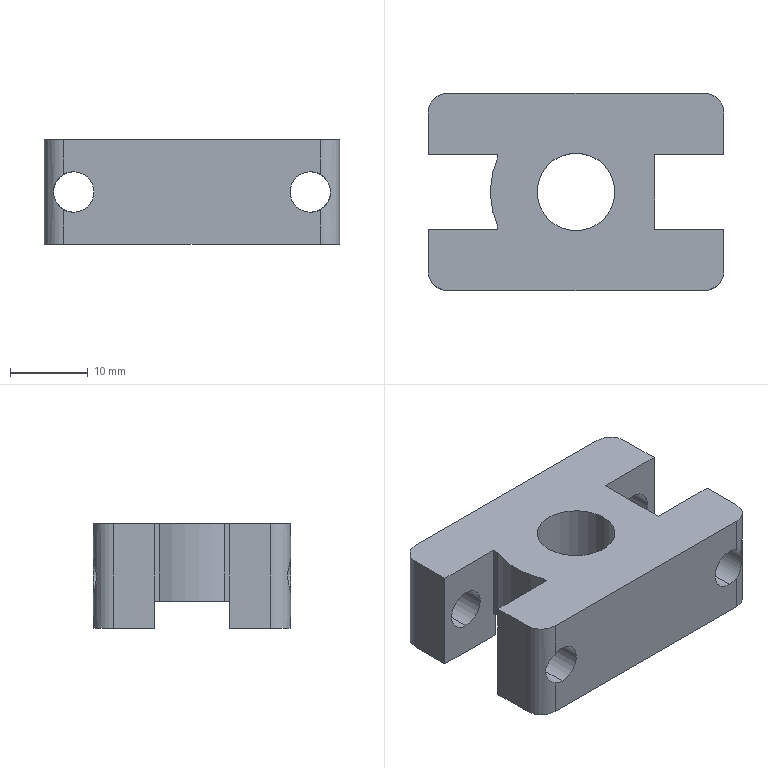Part | SolidWorks | features Cut 2, ICE 2, Extrusion 1, Fillet 1 | 1 solid | 34 faces | box 38.1 x 25.4 x 13.5 mm | volume 7968 mm3 | cylinder 17 | plane 17 | commonest cylinder face diameters 5.207 x8 5.08 x4 22 x3 10 x2
STEP:
#1=CARTESIAN_POINT('',(-15.24,-12.7,0.6465));
#2=VERTEX_POINT('',#1);
#3=CARTESIAN_POINT('',(-16.51,-12.7,0.9773));
#4=VERTEX_POINT('',#3);
#5=CARTESIAN_POINT('',(-15.24,-12.7,3.25));
#6=DIRECTION('',(0.,1.,0.));
#7=DIRECTION('',(0.,0.,1.));
#8=AXIS2_PLACEMENT_3D('',#5,#6,#7);
#9=CIRCLE('',#8,2.604);
#10=EDGE_CURVE('',#2,#4,#9,.T.);
#11=ORIENTED_EDGE('',*,*,#10,.F.);
#12=CARTESIAN_POINT('',(-15.24,-4.826,0.6465));
#13=VERTEX_POINT('',#12);
#14=CARTESIAN_POINT('',(-15.24,-12.7,0.6465));
#15=DIRECTION('',(0.,1.,0.));
#16=VECTOR('',#15,1000.);
#17=LINE('',#14,#16);
#18=EDGE_CURVE('',#2,#13,#17,.T.);
#19=ORIENTED_EDGE('',*,*,#18,.T.);
#20=CARTESIAN_POINT('',(-15.24,-4.826,5.853));
#21=VERTEX_POINT('',#20);
#22=CARTESIAN_POINT('',(-15.24,-4.826,3.25));
#23=DIRECTION('',(0.,1.,0.));
#24=DIRECTION('',(0.,0.,1.));
#25=AXIS2_PLACEMENT_3D('',#22,#23,#24);
#26=CIRCLE('',#25,2.604);
#27=EDGE_CURVE('',#13,#21,#26,.T.);
#28=ORIENTED_EDGE('',*,*,#27,.T.);
#29=CARTESIAN_POINT('',(-15.24,-12.7,5.853));
#30=VERTEX_POINT('',#29);
#31=CARTESIAN_POINT('',(-15.24,-12.7,5.853));
#32=DIRECTION('',(0.,1.,0.));
#33=VECTOR('',#32,1000.);
#34=LINE('',#31,#33);
#35=EDGE_CURVE('',#30,#21,#34,.T.);
#36=ORIENTED_EDGE('',*,*,#35,.F.);
#37=CARTESIAN_POINT('',(-16.51,-12.7,5.523));
#38=VERTEX_POINT('',#37);
#39=CARTESIAN_POINT('',(-15.24,-12.7,3.25));
#40=DIRECTION('',(0.,1.,0.));
#41=DIRECTION('',(0.,0.,1.));
#42=AXIS2_PLACEMENT_3D('',#39,#40,#41);
#43=CIRCLE('',#42,2.604);
#44=EDGE_CURVE('',#38,#30,#43,.T.);
#45=ORIENTED_EDGE('',*,*,#44,.F.);
#46=CARTESIAN_POINT('',(-16.51,-12.7,5.523));
#47=CARTESIAN_POINT('',(-16.715,-12.7,5.408));
#48=CARTESIAN_POINT('',(-16.899,-12.676,5.269));
#49=CARTESIAN_POINT('',(-17.228,-12.602,4.947));
#50=CARTESIAN_POINT('',(-17.369,-12.553,4.765));
#51=CARTESIAN_POINT('',(-17.6,-12.458,4.373));
#52=CARTESIAN_POINT('',(-17.69,-12.41,4.159));
#53=CARTESIAN_POINT('',(-17.781,-12.359,3.829));
#54=CARTESIAN_POINT('',(-17.804,-12.346,3.716));
#55=CARTESIAN_POINT('',(-17.835,-12.327,3.486));
#56=CARTESIAN_POINT('',(-17.843,-12.322,3.368));
#57=CARTESIAN_POINT('',(-17.844,-12.322,3.02));
#58=CARTESIAN_POINT('',(-17.813,-12.342,2.789));
#59=CARTESIAN_POINT('',(-17.691,-12.41,2.342));
#60=CARTESIAN_POINT('',(-17.602,-12.457,2.131));
#61=CARTESIAN_POINT('',(-17.37,-12.553,1.736));
#62=CARTESIAN_POINT('',(-17.231,-12.601,1.557));
#63=CARTESIAN_POINT('',(-16.903,-12.675,1.233));
#64=CARTESIAN_POINT('',(-16.715,-12.7,1.092));
#65=CARTESIAN_POINT('',(-16.51,-12.7,0.9773));
#66=B_SPLINE_CURVE_WITH_KNOTS('',3,(#46,#47,#48,#49,#50,#51,#52,#53,#54,#55,#56,#57,#58,#59,#60,#61,#62,#63,#64,#65),.UNSPECIFIED.,.F.,.F.,(4,2,2,2,2,2,2,2,2,4),(0.,0.000694,0.001388,0.002082,0.002429,0.002776,0.00347,0.004164,0.004858,0.005552),.UNSPECIFIED.);
#67=EDGE_CURVE('',#38,#4,#66,.T.);
#68=ORIENTED_EDGE('',*,*,#67,.T.);
#69=EDGE_LOOP('',(#11,#19,#28,#36,#45,#68));
#70=FACE_OUTER_BOUND('',#69,.T.);
#71=CARTESIAN_POINT('',(-15.24,-12.7,3.25));
#72=DIRECTION('',(0.,1.,0.));
#73=DIRECTION('',(0.,0.,1.));
#74=AXIS2_PLACEMENT_3D('',#71,#72,#73);
#75=CYLINDRICAL_SURFACE('',#74,2.604);
#76=ADVANCED_FACE('',(#70),#75,.F.);
#77=CARTESIAN_POINT('',(-15.24,4.826,0.6465));
#78=VERTEX_POINT('',#77);
#79=CARTESIAN_POINT('',(-15.24,4.826,5.853));
#80=VERTEX_POINT('',#79);
#81=CARTESIAN_POINT('',(-15.24,4.826,3.25));
#82=DIRECTION('',(0.,1.,0.));
#83=DIRECTION('',(0.,0.,1.));
#84=AXIS2_PLACEMENT_3D('',#81,#82,#83);
#85=CIRCLE('',#84,2.604);
#86=EDGE_CURVE('',#78,#80,#85,.T.);
#87=ORIENTED_EDGE('',*,*,#86,.F.);
#88=CARTESIAN_POINT('',(-15.24,12.7,0.6465));
#89=VERTEX_POINT('',#88);
#90=CARTESIAN_POINT('',(-15.24,-12.7,0.6465));
#91=DIRECTION('',(0.,1.,0.));
#92=VECTOR('',#91,1000.);
#93=LINE('',#90,#92);
#94=EDGE_CURVE('',#78,#89,#93,.T.);
#95=ORIENTED_EDGE('',*,*,#94,.T.);
#96=CARTESIAN_POINT('',(-16.51,12.7,0.9773));
#97=VERTEX_POINT('',#96);
#98=CARTESIAN_POINT('',(-15.24,12.7,3.25));
#99=DIRECTION('',(0.,1.,0.));
#100=DIRECTION('',(0.,0.,1.));
#101=AXIS2_PLACEMENT_3D('',#98,#99,#100);
#102=CIRCLE('',#101,2.604);
#103=EDGE_CURVE('',#89,#97,#102,.T.);
#104=ORIENTED_EDGE('',*,*,#103,.T.);
#105=CARTESIAN_POINT('',(-16.51,12.7,5.523));
#106=VERTEX_POINT('',#105);
#107=CARTESIAN_POINT('',(-16.51,12.7,0.9773));
#108=CARTESIAN_POINT('',(-16.715,12.7,1.092));
#109=CARTESIAN_POINT('',(-16.899,12.676,1.231));
#110=CARTESIAN_POINT('',(-17.228,12.602,1.553));
#111=CARTESIAN_POINT('',(-17.369,12.553,1.735));
#112=CARTESIAN_POINT('',(-17.6,12.458,2.127));
#113=CARTESIAN_POINT('',(-17.69,12.41,2.341));
#114=CARTESIAN_POINT('',(-17.781,12.359,2.671));
#115=CARTESIAN_POINT('',(-17.804,12.346,2.784));
#116=CARTESIAN_POINT('',(-17.835,12.327,3.014));
#117=CARTESIAN_POINT('',(-17.843,12.322,3.132));
#118=CARTESIAN_POINT('',(-17.844,12.322,3.48));
#119=CARTESIAN_POINT('',(-17.813,12.342,3.711));
#120=CARTESIAN_POINT('',(-17.691,12.41,4.158));
#121=CARTESIAN_POINT('',(-17.602,12.457,4.369));
#122=CARTESIAN_POINT('',(-17.37,12.553,4.764));
#123=CARTESIAN_POINT('',(-17.231,12.601,4.943));
#124=CARTESIAN_POINT('',(-16.903,12.675,5.267));
#125=CARTESIAN_POINT('',(-16.715,12.7,5.408));
#126=CARTESIAN_POINT('',(-16.51,12.7,5.523));
#127=B_SPLINE_CURVE_WITH_KNOTS('',3,(#107,#108,#109,#110,#111,#112,#113,#114,#115,#116,#117,#118,#119,#120,#121,#122,#123,#124,#125,#126),.UNSPECIFIED.,.F.,.F.,(4,2,2,2,2,2,2,2,2,4),(0.,0.000694,0.001388,0.002082,0.002429,0.002776,0.00347,0.004164,0.004858,0.005552),.UNSPECIFIED.);
#128=EDGE_CURVE('',#97,#106,#127,.T.);
#129=ORIENTED_EDGE('',*,*,#128,.T.);
#130=CARTESIAN_POINT('',(-15.24,12.7,5.853));
#131=VERTEX_POINT('',#130);
#132=CARTESIAN_POINT('',(-15.24,12.7,3.25));
#133=DIRECTION('',(0.,1.,0.));
#134=DIRECTION('',(0.,0.,1.));
#135=AXIS2_PLACEMENT_3D('',#132,#133,#134);
#136=CIRCLE('',#135,2.604);
#137=EDGE_CURVE('',#106,#131,#136,.T.);
#138=ORIENTED_EDGE('',*,*,#137,.T.);
#139=CARTESIAN_POINT('',(-15.24,-12.7,5.853));
#140=DIRECTION('',(0.,1.,0.));
#141=VECTOR('',#140,1000.);
#142=LINE('',#139,#141);
#143=EDGE_CURVE('',#80,#131,#142,.T.);
#144=ORIENTED_EDGE('',*,*,#143,.F.);
#145=EDGE_LOOP('',(#87,#95,#104,#129,#138,#144));
#146=FACE_OUTER_BOUND('',#145,.T.);
#147=CARTESIAN_POINT('',(-15.24,-12.7,3.25));
#148=DIRECTION('',(0.,1.,0.));
#149=DIRECTION('',(0.,0.,1.));
#150=AXIS2_PLACEMENT_3D('',#147,#148,#149);
#151=CYLINDRICAL_SURFACE('',#150,2.604);
#152=ADVANCED_FACE('',(#146),#151,.F.);
#153=CARTESIAN_POINT('',(15.24,4.826,5.854));
#154=VERTEX_POINT('',#153);
#155=CARTESIAN_POINT('',(15.24,4.826,0.6465));
#156=VERTEX_POINT('',#155);
#157=CARTESIAN_POINT('',(15.24,4.826,3.25));
#158=DIRECTION('',(0.,-1.,0.));
#159=DIRECTION('',(0.,0.,-1.));
#160=AXIS2_PLACEMENT_3D('',#157,#158,#159);
#161=CIRCLE('',#160,2.604);
#162=EDGE_CURVE('',#154,#156,#161,.T.);
#163=ORIENTED_EDGE('',*,*,#162,.T.);
#164=CARTESIAN_POINT('',(15.24,12.7,0.6465));
#165=VERTEX_POINT('',#164);
#166=CARTESIAN_POINT('',(15.24,-12.7,0.6465));
#167=DIRECTION('',(0.,1.,0.));
#168=VECTOR('',#167,1000.);
#169=LINE('',#166,#168);
#170=EDGE_CURVE('',#156,#165,#169,.T.);
#171=ORIENTED_EDGE('',*,*,#170,.T.);
#172=CARTESIAN_POINT('',(15.24,12.7,5.854));
#173=VERTEX_POINT('',#172);
#174=CARTESIAN_POINT('',(15.24,12.7,3.25));
#175=DIRECTION('',(0.,1.,0.));
#176=DIRECTION('',(0.,0.,1.));
#177=AXIS2_PLACEMENT_3D('',#174,#175,#176);
#178=CIRCLE('',#177,2.604);
#179=EDGE_CURVE('',#165,#173,#178,.T.);
#180=ORIENTED_EDGE('',*,*,#179,.T.);
#181=CARTESIAN_POINT('',(15.24,-12.7,5.854));
#182=DIRECTION('',(0.,1.,0.));
#183=VECTOR('',#182,1000.);
#184=LINE('',#181,#183);
#185=EDGE_CURVE('',#154,#173,#184,.T.);
#186=ORIENTED_EDGE('',*,*,#185,.F.);
#187=EDGE_LOOP('',(#163,#171,#180,#186));
#188=FACE_OUTER_BOUND('',#187,.T.);
#189=CARTESIAN_POINT('',(15.24,-12.7,3.25));
#190=DIRECTION('',(0.,1.,0.));
#191=DIRECTION('',(0.,0.,1.));
#192=AXIS2_PLACEMENT_3D('',#189,#190,#191);
#193=CYLINDRICAL_SURFACE('',#192,2.604);
#194=ADVANCED_FACE('',(#188),#193,.F.);
#195=CARTESIAN_POINT('',(15.24,-12.7,0.6465));
#196=VERTEX_POINT('',#195);
#197=CARTESIAN_POINT('',(15.24,-12.7,5.854));
#198=VERTEX_POINT('',#197);
#199=CARTESIAN_POINT('',(15.24,-12.7,3.25));
#200=DIRECTION('',(0.,1.,0.));
#201=DIRECTION('',(0.,0.,1.));
#202=AXIS2_PLACEMENT_3D('',#199,#200,#201);
#203=CIRCLE('',#202,2.604);
#204=EDGE_CURVE('',#196,#198,#203,.T.);
#205=ORIENTED_EDGE('',*,*,#204,.F.);
#206=CARTESIAN_POINT('',(15.24,-4.826,0.6465));
#207=VERTEX_POINT('',#206);
#208=CARTESIAN_POINT('',(15.24,-12.7,0.6465));
#209=DIRECTION('',(0.,1.,0.));
#210=VECTOR('',#209,1000.);
#211=LINE('',#208,#210);
#212=EDGE_CURVE('',#196,#207,#211,.T.);
#213=ORIENTED_EDGE('',*,*,#212,.T.);
#214=CARTESIAN_POINT('',(15.24,-4.826,5.854));
#215=VERTEX_POINT('',#214);
#216=CARTESIAN_POINT('',(15.24,-4.826,3.25));
#217=DIRECTION('',(0.,-1.,0.));
#218=DIRECTION('',(0.,0.,-1.));
#219=AXIS2_PLACEMENT_3D('',#216,#217,#218);
#220=CIRCLE('',#219,2.604);
#221=EDGE_CURVE('',#215,#207,#220,.T.);
#222=ORIENTED_EDGE('',*,*,#221,.F.);
#223=CARTESIAN_POINT('',(15.24,-12.7,5.854));
#224=DIRECTION('',(0.,1.,0.));
#225=VECTOR('',#224,1000.);
#226=LINE('',#223,#225);
#227=EDGE_CURVE('',#198,#215,#226,.T.);
#228=ORIENTED_EDGE('',*,*,#227,.F.);
#229=EDGE_LOOP('',(#205,#213,#222,#228));
#230=FACE_OUTER_BOUND('',#229,.T.);
#231=CARTESIAN_POINT('',(15.24,-12.7,3.25));
#232=DIRECTION('',(0.,1.,0.));
#233=DIRECTION('',(0.,0.,1.));
#234=AXIS2_PLACEMENT_3D('',#231,#232,#233);
#235=CYLINDRICAL_SURFACE('',#234,2.604);
#236=ADVANCED_FACE('',(#230),#235,.F.);
#237=CARTESIAN_POINT('',(-5.,0.,0.));
#238=VERTEX_POINT('',#237);
#239=CARTESIAN_POINT('',(5.,0.,0.));
#240=VERTEX_POINT('',#239);
#241=CARTESIAN_POINT('',(0.,0.,0.));
#242=DIRECTION('',(0.,0.,1.));
#243=DIRECTION('',(0.,-1.,0.));
#244=AXIS2_PLACEMENT_3D('',#241,#242,#243);
#245=CIRCLE('',#244,5.);
#246=EDGE_CURVE('',#238,#240,#245,.T.);
#247=ORIENTED_EDGE('',*,*,#246,.F.);
#248=CARTESIAN_POINT('',(-5.,0.,10.));
#249=VERTEX_POINT('',#248);
#250=CARTESIAN_POINT('',(-5.,0.,-31.113));
#251=DIRECTION('',(0.,0.,1.));
#252=VECTOR('',#251,1000.);
#253=LINE('',#250,#252);
#254=EDGE_CURVE('',#238,#249,#253,.T.);
#255=ORIENTED_EDGE('',*,*,#254,.T.);
#256=CARTESIAN_POINT('',(5.,0.,10.));
#257=VERTEX_POINT('',#256);
#258=CARTESIAN_POINT('',(0.,0.,10.));
#259=DIRECTION('',(0.,0.,1.));
#260=DIRECTION('',(1.,0.,0.));
#261=AXIS2_PLACEMENT_3D('',#258,#259,#260);
#262=CIRCLE('',#261,5.);
#263=EDGE_CURVE('',#249,#257,#262,.T.);
#264=ORIENTED_EDGE('',*,*,#263,.T.);
#265=CARTESIAN_POINT('',(5.,0.,-31.113));
#266=DIRECTION('',(0.,0.,1.));
#267=VECTOR('',#266,1000.);
#268=LINE('',#265,#267);
#269=EDGE_CURVE('',#240,#257,#268,.T.);
#270=ORIENTED_EDGE('',*,*,#269,.F.);
#271=EDGE_LOOP('',(#247,#255,#264,#270));
#272=FACE_OUTER_BOUND('',#271,.T.);
#273=CARTESIAN_POINT('',(0.,0.,-31.113));
#274=DIRECTION('',(0.,0.,1.));
#275=DIRECTION('',(1.,0.,0.));
#276=AXIS2_PLACEMENT_3D('',#273,#274,#275);
#277=CYLINDRICAL_SURFACE('',#276,5.);
#278=ADVANCED_FACE('',(#272),#277,.F.);
#279=CARTESIAN_POINT('',(9.885,4.826,0.));
#280=VERTEX_POINT('',#279);
#281=CARTESIAN_POINT('',(9.885,4.826,-3.5));
#282=VERTEX_POINT('',#281);
#283=CARTESIAN_POINT('',(9.885,4.826,55.791));
#284=DIRECTION('',(0.,0.,-1.));
#285=VECTOR('',#284,1000.);
#286=LINE('',#283,#285);
#287=EDGE_CURVE('',#280,#282,#286,.T.);
#288=ORIENTED_EDGE('',*,*,#287,.F.);
#289=CARTESIAN_POINT('',(-9.885,4.826,0.));
#290=VERTEX_POINT('',#289);
#291=CARTESIAN_POINT('',(0.,0.,0.));
#292=DIRECTION('',(0.,0.,1.));
#293=DIRECTION('',(0.,-1.,0.));
#294=AXIS2_PLACEMENT_3D('',#291,#292,#293);
#295=CIRCLE('',#294,11.);
#296=EDGE_CURVE('',#280,#290,#295,.T.);
#297=ORIENTED_EDGE('',*,*,#296,.T.);
#298=CARTESIAN_POINT('',(-9.885,4.826,-3.5));
#299=VERTEX_POINT('',#298);
#300=CARTESIAN_POINT('',(-9.885,4.826,55.791));
#301=DIRECTION('',(0.,0.,1.));
#302=VECTOR('',#301,1000.);
#303=LINE('',#300,#302);
#304=EDGE_CURVE('',#299,#290,#303,.T.);
#305=ORIENTED_EDGE('',*,*,#304,.F.);
#306=CARTESIAN_POINT('',(0.,0.,-3.5));
#307=DIRECTION('',(0.,0.,-1.));
#308=DIRECTION('',(0.,-1.,0.));
#309=AXIS2_PLACEMENT_3D('',#306,#307,#308);
#310=CIRCLE('',#309,11.);
#311=EDGE_CURVE('',#299,#282,#310,.T.);
#312=ORIENTED_EDGE('',*,*,#311,.T.);
#313=EDGE_LOOP('',(#288,#297,#305,#312));
#314=FACE_OUTER_BOUND('',#313,.T.);
#315=CARTESIAN_POINT('',(0.,0.,55.791));
#316=DIRECTION('',(0.,0.,-1.));
#317=DIRECTION('',(-1.,0.,0.));
#318=AXIS2_PLACEMENT_3D('',#315,#316,#317);
#319=CYLINDRICAL_SURFACE('',#318,11.);
#320=ADVANCED_FACE('',(#314),#319,.F.);
#321=CARTESIAN_POINT('',(0.,0.,10.));
#322=DIRECTION('',(0.,0.,1.));
#323=DIRECTION('',(1.,0.,0.));
#324=AXIS2_PLACEMENT_3D('',#321,#322,#323);
#325=CIRCLE('',#324,5.);
#326=EDGE_CURVE('',#257,#249,#325,.T.);
#327=ORIENTED_EDGE('',*,*,#326,.F.);
#328=ORIENTED_EDGE('',*,*,#263,.F.);
#329=EDGE_LOOP('',(#327,#328));
#330=FACE_BOUND('',#329,.T.);
#331=CARTESIAN_POINT('',(-19.05,-10.16,10.));
#332=VERTEX_POINT('',#331);
#333=CARTESIAN_POINT('',(-19.05,-4.826,10.));
#334=VERTEX_POINT('',#333);
#335=CARTESIAN_POINT('',(-19.05,0.,10.));
#336=DIRECTION('',(0.,1.,0.));
#337=VECTOR('',#336,1000.);
#338=LINE('',#335,#337);
#339=EDGE_CURVE('',#332,#334,#338,.T.);
#340=ORIENTED_EDGE('',*,*,#339,.F.);
#341=CARTESIAN_POINT('',(-16.51,-12.7,10.));
#342=VERTEX_POINT('',#341);
#343=CARTESIAN_POINT('',(-16.51,-10.16,10.));
#344=DIRECTION('',(0.,0.,1.));
#345=DIRECTION('',(0.,-1.,0.));
#346=AXIS2_PLACEMENT_3D('',#343,#344,#345);
#347=CIRCLE('',#346,2.54);
#348=EDGE_CURVE('',#332,#342,#347,.T.);
#349=ORIENTED_EDGE('',*,*,#348,.T.);
#350=CARTESIAN_POINT('',(16.51,-12.7,10.));
#351=VERTEX_POINT('',#350);
#352=CARTESIAN_POINT('',(0.,-12.7,10.));
#353=DIRECTION('',(1.,0.,0.));
#354=VECTOR('',#353,1000.);
#355=LINE('',#352,#354);
#356=EDGE_CURVE('',#342,#351,#355,.T.);
#357=ORIENTED_EDGE('',*,*,#356,.T.);
#358=CARTESIAN_POINT('',(19.05,-10.16,10.));
#359=VERTEX_POINT('',#358);
#360=CARTESIAN_POINT('',(16.51,-10.16,10.));
#361=DIRECTION('',(0.,0.,1.));
#362=DIRECTION('',(0.,-1.,0.));
#363=AXIS2_PLACEMENT_3D('',#360,#361,#362);
#364=CIRCLE('',#363,2.54);
#365=EDGE_CURVE('',#351,#359,#364,.T.);
#366=ORIENTED_EDGE('',*,*,#365,.T.);
#367=CARTESIAN_POINT('',(19.05,-4.826,10.));
#368=VERTEX_POINT('',#367);
#369=CARTESIAN_POINT('',(19.05,0.,10.));
#370=DIRECTION('',(0.,1.,0.));
#371=VECTOR('',#370,1000.);
#372=LINE('',#369,#371);
#373=EDGE_CURVE('',#359,#368,#372,.T.);
#374=ORIENTED_EDGE('',*,*,#373,.T.);
#375=CARTESIAN_POINT('',(10.16,-4.826,10.));
#376=VERTEX_POINT('',#375);
#377=CARTESIAN_POINT('',(27.94,-4.826,10.));
#378=DIRECTION('',(-1.,0.,0.));
#379=VECTOR('',#378,1000.);
#380=LINE('',#377,#379);
#381=EDGE_CURVE('',#368,#376,#380,.T.);
#382=ORIENTED_EDGE('',*,*,#381,.T.);
#383=CARTESIAN_POINT('',(10.16,4.826,10.));
#384=VERTEX_POINT('',#383);
#385=CARTESIAN_POINT('',(10.16,-4.826,10.));
#386=DIRECTION('',(0.,1.,0.));
#387=VECTOR('',#386,1000.);
#388=LINE('',#385,#387);
#389=EDGE_CURVE('',#376,#384,#388,.T.);
#390=ORIENTED_EDGE('',*,*,#389,.T.);
#391=CARTESIAN_POINT('',(19.05,4.826,10.));
#392=VERTEX_POINT('',#391);
#393=CARTESIAN_POINT('',(27.94,4.826,10.));
#394=DIRECTION('',(-1.,0.,0.));
#395=VECTOR('',#394,1000.);
#396=LINE('',#393,#395);
#397=EDGE_CURVE('',#392,#384,#396,.T.);
#398=ORIENTED_EDGE('',*,*,#397,.F.);
#399=CARTESIAN_POINT('',(19.05,10.16,10.));
#400=VERTEX_POINT('',#399);
#401=CARTESIAN_POINT('',(19.05,0.,10.));
#402=DIRECTION('',(0.,1.,0.));
#403=VECTOR('',#402,1000.);
#404=LINE('',#401,#403);
#405=EDGE_CURVE('',#392,#400,#404,.T.);
#406=ORIENTED_EDGE('',*,*,#405,.T.);
#407=CARTESIAN_POINT('',(16.51,12.7,10.));
#408=VERTEX_POINT('',#407);
#409=CARTESIAN_POINT('',(16.51,10.16,10.));
#410=DIRECTION('',(0.,0.,1.));
#411=DIRECTION('',(0.,-1.,0.));
#412=AXIS2_PLACEMENT_3D('',#409,#410,#411);
#413=CIRCLE('',#412,2.54);
#414=EDGE_CURVE('',#400,#408,#413,.T.);
#415=ORIENTED_EDGE('',*,*,#414,.T.);
#416=CARTESIAN_POINT('',(-16.51,12.7,10.));
#417=VERTEX_POINT('',#416);
#418=CARTESIAN_POINT('',(0.,12.7,10.));
#419=DIRECTION('',(1.,0.,0.));
#420=VECTOR('',#419,1000.);
#421=LINE('',#418,#420);
#422=EDGE_CURVE('',#417,#408,#421,.T.);
#423=ORIENTED_EDGE('',*,*,#422,.F.);
#424=CARTESIAN_POINT('',(-19.05,10.16,10.));
#425=VERTEX_POINT('',#424);
#426=CARTESIAN_POINT('',(-16.51,10.16,10.));
#427=DIRECTION('',(0.,0.,1.));
#428=DIRECTION('',(0.,-1.,0.));
#429=AXIS2_PLACEMENT_3D('',#426,#427,#428);
#430=CIRCLE('',#429,2.54);
#431=EDGE_CURVE('',#417,#425,#430,.T.);
#432=ORIENTED_EDGE('',*,*,#431,.T.);
#433=CARTESIAN_POINT('',(-19.05,4.826,10.));
#434=VERTEX_POINT('',#433);
#435=CARTESIAN_POINT('',(-19.05,0.,10.));
#436=DIRECTION('',(0.,1.,0.));
#437=VECTOR('',#436,1000.);
#438=LINE('',#435,#437);
#439=EDGE_CURVE('',#434,#425,#438,.T.);
#440=ORIENTED_EDGE('',*,*,#439,.F.);
#441=CARTESIAN_POINT('',(-10.16,4.826,10.));
#442=VERTEX_POINT('',#441);
#443=CARTESIAN_POINT('',(0.,4.826,10.));
#444=DIRECTION('',(1.,0.,0.));
#445=VECTOR('',#444,1000.);
#446=LINE('',#443,#445);
#447=EDGE_CURVE('',#434,#442,#446,.T.);
#448=ORIENTED_EDGE('',*,*,#447,.T.);
#449=CARTESIAN_POINT('',(-10.16,4.216,10.));
#450=VERTEX_POINT('',#449);
#451=CARTESIAN_POINT('',(-10.16,0.,10.));
#452=DIRECTION('',(0.,1.,0.));
#453=VECTOR('',#452,1000.);
#454=LINE('',#451,#453);
#455=EDGE_CURVE('',#450,#442,#454,.T.);
#456=ORIENTED_EDGE('',*,*,#455,.F.);
#457=CARTESIAN_POINT('',(-10.16,-4.216,10.));
#458=VERTEX_POINT('',#457);
#459=CARTESIAN_POINT('',(0.,0.,10.));
#460=DIRECTION('',(0.,0.,1.));
#461=DIRECTION('',(-1.,0.,0.));
#462=AXIS2_PLACEMENT_3D('',#459,#460,#461);
#463=CIRCLE('',#462,11.);
#464=EDGE_CURVE('',#450,#458,#463,.T.);
#465=ORIENTED_EDGE('',*,*,#464,.T.);
#466=CARTESIAN_POINT('',(-10.16,-4.826,10.));
#467=VERTEX_POINT('',#466);
#468=CARTESIAN_POINT('',(-10.16,0.,10.));
#469=DIRECTION('',(0.,1.,0.));
#470=VECTOR('',#469,1000.);
#471=LINE('',#468,#470);
#472=EDGE_CURVE('',#467,#458,#471,.T.);
#473=ORIENTED_EDGE('',*,*,#472,.F.);
#474=CARTESIAN_POINT('',(0.,-4.826,10.));
#475=DIRECTION('',(1.,0.,0.));
#476=VECTOR('',#475,1000.);
#477=LINE('',#474,#476);
#478=EDGE_CURVE('',#334,#467,#477,.T.);
#479=ORIENTED_EDGE('',*,*,#478,.F.);
#480=EDGE_LOOP('',(#340,#349,#357,#366,#374,#382,#390,#398,#406,#415,#423,#432,#440,#448,#456,#465,#473,#479));
#481=FACE_OUTER_BOUND('',#480,.T.);
#482=CARTESIAN_POINT('',(0.,0.,10.));
#483=DIRECTION('',(0.,0.,1.));
#484=DIRECTION('',(0.,-1.,0.));
#485=AXIS2_PLACEMENT_3D('',#482,#483,#484);
#486=PLANE('',#485);
#487=ADVANCED_FACE('',(#330,#481),#486,.T.);
#488=CARTESIAN_POINT('',(-19.05,10.16,-3.5));
#489=VERTEX_POINT('',#488);
#490=CARTESIAN_POINT('',(-19.05,4.826,-3.5));
#491=VERTEX_POINT('',#490);
#492=CARTESIAN_POINT('',(-19.05,0.,-3.5));
#493=DIRECTION('',(0.,-1.,0.));
#494=VECTOR('',#493,1000.);
#495=LINE('',#492,#494);
#496=EDGE_CURVE('',#489,#491,#495,.T.);
#497=ORIENTED_EDGE('',*,*,#496,.F.);
#498=CARTESIAN_POINT('',(-16.51,12.7,-3.5));
#499=VERTEX_POINT('',#498);
#500=CARTESIAN_POINT('',(-16.51,10.16,-3.5));
#501=DIRECTION('',(0.,0.,-1.));
#502=DIRECTION('',(0.,-1.,0.));
#503=AXIS2_PLACEMENT_3D('',#500,#501,#502);
#504=CIRCLE('',#503,2.54);
#505=EDGE_CURVE('',#489,#499,#504,.T.);
#506=ORIENTED_EDGE('',*,*,#505,.T.);
#507=CARTESIAN_POINT('',(16.51,12.7,-3.5));
#508=VERTEX_POINT('',#507);
#509=CARTESIAN_POINT('',(0.,12.7,-3.5));
#510=DIRECTION('',(-1.,0.,0.));
#511=VECTOR('',#510,1000.);
#512=LINE('',#509,#511);
#513=EDGE_CURVE('',#508,#499,#512,.T.);
#514=ORIENTED_EDGE('',*,*,#513,.F.);
#515=CARTESIAN_POINT('',(19.05,10.16,-3.5));
#516=VERTEX_POINT('',#515);
#517=CARTESIAN_POINT('',(16.51,10.16,-3.5));
#518=DIRECTION('',(0.,0.,-1.));
#519=DIRECTION('',(0.,-1.,0.));
#520=AXIS2_PLACEMENT_3D('',#517,#518,#519);
#521=CIRCLE('',#520,2.54);
#522=EDGE_CURVE('',#508,#516,#521,.T.);
#523=ORIENTED_EDGE('',*,*,#522,.T.);
#524=CARTESIAN_POINT('',(19.05,4.826,-3.5));
#525=VERTEX_POINT('',#524);
#526=CARTESIAN_POINT('',(19.05,0.,-3.5));
#527=DIRECTION('',(0.,-1.,0.));
#528=VECTOR('',#527,1000.);
#529=LINE('',#526,#528);
#530=EDGE_CURVE('',#516,#525,#529,.T.);
#531=ORIENTED_EDGE('',*,*,#530,.T.);
#532=CARTESIAN_POINT('',(27.94,4.826,-3.5));
#533=DIRECTION('',(-1.,0.,0.));
#534=VECTOR('',#533,1000.);
#535=LINE('',#532,#534);
#536=EDGE_CURVE('',#525,#282,#535,.T.);
#537=ORIENTED_EDGE('',*,*,#536,.T.);
#538=ORIENTED_EDGE('',*,*,#311,.F.);
#539=CARTESIAN_POINT('',(0.,4.826,-3.5));
#540=DIRECTION('',(-1.,0.,0.));
#541=VECTOR('',#540,1000.);
#542=LINE('',#539,#541);
#543=EDGE_CURVE('',#299,#491,#542,.T.);
#544=ORIENTED_EDGE('',*,*,#543,.T.);
#545=EDGE_LOOP('',(#497,#506,#514,#523,#531,#537,#538,#544));
#546=FACE_OUTER_BOUND('',#545,.T.);
#547=CARTESIAN_POINT('',(0.,0.,-3.5));
#548=DIRECTION('',(0.,0.,1.));
#549=DIRECTION('',(0.,-1.,0.));
#550=AXIS2_PLACEMENT_3D('',#547,#548,#549);
#551=PLANE('',#550);
#552=ADVANCED_FACE('',(#546),#551,.F.);
#553=ORIENTED_EDGE('',*,*,#530,.F.);
#554=CARTESIAN_POINT('',(19.05,10.16,10.));
#555=DIRECTION('',(0.,0.,1.));
#556=VECTOR('',#555,1000.);
#557=LINE('',#554,#556);
#558=EDGE_CURVE('',#516,#400,#557,.T.);
#559=ORIENTED_EDGE('',*,*,#558,.T.);
#560=ORIENTED_EDGE('',*,*,#405,.F.);
#561=CARTESIAN_POINT('',(19.05,4.826,55.791));
#562=DIRECTION('',(0.,0.,1.));
#563=VECTOR('',#562,1000.);
#564=LINE('',#561,#563);
#565=EDGE_CURVE('',#525,#392,#564,.T.);
#566=ORIENTED_EDGE('',*,*,#565,.F.);
#567=EDGE_LOOP('',(#553,#559,#560,#566));
#568=FACE_OUTER_BOUND('',#567,.T.);
#569=CARTESIAN_POINT('',(19.05,0.,55.791));
#570=DIRECTION('',(-1.,0.,0.));
#571=DIRECTION('',(0.,0.,1.));
#572=AXIS2_PLACEMENT_3D('',#569,#570,#571);
#573=PLANE('',#572);
#574=ADVANCED_FACE('',(#568),#573,.F.);
#575=CARTESIAN_POINT('',(-9.885,-4.826,0.));
#576=VERTEX_POINT('',#575);
#577=CARTESIAN_POINT('',(-9.885,-4.826,-3.5));
#578=VERTEX_POINT('',#577);
#579=CARTESIAN_POINT('',(-9.885,-4.826,55.791));
#580=DIRECTION('',(0.,0.,-1.));
#581=VECTOR('',#580,1000.);
#582=LINE('',#579,#581);
#583=EDGE_CURVE('',#576,#578,#582,.T.);
#584=ORIENTED_EDGE('',*,*,#583,.F.);
#585=CARTESIAN_POINT('',(9.885,-4.826,0.));
#586=VERTEX_POINT('',#585);
#587=CARTESIAN_POINT('',(0.,0.,0.));
#588=DIRECTION('',(0.,0.,1.));
#589=DIRECTION('',(0.,-1.,0.));
#590=AXIS2_PLACEMENT_3D('',#587,#588,#589);
#591=CIRCLE('',#590,11.);
#592=EDGE_CURVE('',#576,#586,#591,.T.);
#593=ORIENTED_EDGE('',*,*,#592,.T.);
#594=CARTESIAN_POINT('',(9.885,-4.826,-3.5));
#595=VERTEX_POINT('',#594);
#596=CARTESIAN_POINT('',(9.885,-4.826,55.791));
#597=DIRECTION('',(0.,0.,1.));
#598=VECTOR('',#597,1000.);
#599=LINE('',#596,#598);
#600=EDGE_CURVE('',#595,#586,#599,.T.);
#601=ORIENTED_EDGE('',*,*,#600,.F.);
#602=CARTESIAN_POINT('',(0.,0.,-3.5));
#603=DIRECTION('',(0.,0.,-1.));
#604=DIRECTION('',(0.,-1.,0.));
#605=AXIS2_PLACEMENT_3D('',#602,#603,#604);
#606=CIRCLE('',#605,11.);
#607=EDGE_CURVE('',#595,#578,#606,.T.);
#608=ORIENTED_EDGE('',*,*,#607,.T.);
#609=EDGE_LOOP('',(#584,#593,#601,#608));
#610=FACE_OUTER_BOUND('',#609,.T.);
#611=CARTESIAN_POINT('',(0.,0.,55.791));
#612=DIRECTION('',(0.,0.,-1.));
#613=DIRECTION('',(-1.,0.,0.));
#614=AXIS2_PLACEMENT_3D('',#611,#612,#613);
#615=CYLINDRICAL_SURFACE('',#614,11.);
#616=ADVANCED_FACE('',(#610),#615,.F.);
#617=CARTESIAN_POINT('',(-19.05,-4.826,-3.5));
#618=VERTEX_POINT('',#617);
#619=CARTESIAN_POINT('',(-19.05,-10.16,-3.5));
#620=VERTEX_POINT('',#619);
#621=CARTESIAN_POINT('',(-19.05,0.,-3.5));
#622=DIRECTION('',(0.,-1.,0.));
#623=VECTOR('',#622,1000.);
#624=LINE('',#621,#623);
#625=EDGE_CURVE('',#618,#620,#624,.T.);
#626=ORIENTED_EDGE('',*,*,#625,.T.);
#627=CARTESIAN_POINT('',(-19.05,-10.16,10.));
#628=DIRECTION('',(0.,0.,1.));
#629=VECTOR('',#628,1000.);
#630=LINE('',#627,#629);
#631=EDGE_CURVE('',#620,#332,#630,.T.);
#632=ORIENTED_EDGE('',*,*,#631,.T.);
#633=ORIENTED_EDGE('',*,*,#339,.T.);
#634=CARTESIAN_POINT('',(-19.05,-4.826,55.791));
#635=DIRECTION('',(0.,0.,-1.));
#636=VECTOR('',#635,1000.);
#637=LINE('',#634,#636);
#638=EDGE_CURVE('',#334,#618,#637,.T.);
#639=ORIENTED_EDGE('',*,*,#638,.T.);
#640=EDGE_LOOP('',(#626,#632,#633,#639));
#641=FACE_OUTER_BOUND('',#640,.T.);
#642=CARTESIAN_POINT('',(-19.05,0.,55.791));
#643=DIRECTION('',(-1.,0.,0.));
#644=DIRECTION('',(0.,0.,1.));
#645=AXIS2_PLACEMENT_3D('',#642,#643,#644);
#646=PLANE('',#645);
#647=ADVANCED_FACE('',(#641),#646,.T.);
#648=CARTESIAN_POINT('',(16.51,-12.7,-3.5));
#649=VERTEX_POINT('',#648);
#650=CARTESIAN_POINT('',(-16.51,-12.7,-3.5));
#651=VERTEX_POINT('',#650);
#652=CARTESIAN_POINT('',(0.,-12.7,-3.5));
#653=DIRECTION('',(-1.,0.,0.));
#654=VECTOR('',#653,1000.);
#655=LINE('',#652,#654);
#656=EDGE_CURVE('',#649,#651,#655,.T.);
#657=ORIENTED_EDGE('',*,*,#656,.T.);
#658=CARTESIAN_POINT('',(-16.51,-10.16,-3.5));
#659=DIRECTION('',(0.,0.,-1.));
#660=DIRECTION('',(0.,-1.,0.));
#661=AXIS2_PLACEMENT_3D('',#658,#659,#660);
#662=CIRCLE('',#661,2.54);
#663=EDGE_CURVE('',#651,#620,#662,.T.);
#664=ORIENTED_EDGE('',*,*,#663,.T.);
#665=ORIENTED_EDGE('',*,*,#625,.F.);
#666=CARTESIAN_POINT('',(0.,-4.826,-3.5));
#667=DIRECTION('',(-1.,0.,0.));
#668=VECTOR('',#667,1000.);
#669=LINE('',#666,#668);
#670=EDGE_CURVE('',#578,#618,#669,.T.);
#671=ORIENTED_EDGE('',*,*,#670,.F.);
#672=ORIENTED_EDGE('',*,*,#607,.F.);
#673=CARTESIAN_POINT('',(19.05,-4.826,-3.5));
#674=VERTEX_POINT('',#673);
#675=CARTESIAN_POINT('',(27.94,-4.826,-3.5));
#676=DIRECTION('',(-1.,0.,0.));
#677=VECTOR('',#676,1000.);
#678=LINE('',#675,#677);
#679=EDGE_CURVE('',#674,#595,#678,.T.);
#680=ORIENTED_EDGE('',*,*,#679,.F.);
#681=CARTESIAN_POINT('',(19.05,-10.16,-3.5));
#682=VERTEX_POINT('',#681);
#683=CARTESIAN_POINT('',(19.05,0.,-3.5));
#684=DIRECTION('',(0.,-1.,0.));
#685=VECTOR('',#684,1000.);
#686=LINE('',#683,#685);
#687=EDGE_CURVE('',#674,#682,#686,.T.);
#688=ORIENTED_EDGE('',*,*,#687,.T.);
#689=CARTESIAN_POINT('',(16.51,-10.16,-3.5));
#690=DIRECTION('',(0.,0.,-1.));
#691=DIRECTION('',(0.,-1.,0.));
#692=AXIS2_PLACEMENT_3D('',#689,#690,#691);
#693=CIRCLE('',#692,2.54);
#694=EDGE_CURVE('',#682,#649,#693,.T.);
#695=ORIENTED_EDGE('',*,*,#694,.T.);
#696=EDGE_LOOP('',(#657,#664,#665,#671,#672,#680,#688,#695));
#697=FACE_OUTER_BOUND('',#696,.T.);
#698=CARTESIAN_POINT('',(0.,0.,-3.5));
#699=DIRECTION('',(0.,0.,1.));
#700=DIRECTION('',(0.,-1.,0.));
#701=AXIS2_PLACEMENT_3D('',#698,#699,#700);
#702=PLANE('',#701);
#703=ADVANCED_FACE('',(#697),#702,.F.);
#704=ORIENTED_EDGE('',*,*,#439,.T.);
#705=CARTESIAN_POINT('',(-19.05,10.16,55.791));
#706=DIRECTION('',(0.,0.,-1.));
#707=VECTOR('',#706,1000.);
#708=LINE('',#705,#707);
#709=EDGE_CURVE('',#425,#489,#708,.T.);
#710=ORIENTED_EDGE('',*,*,#709,.T.);
#711=ORIENTED_EDGE('',*,*,#496,.T.);
#712=CARTESIAN_POINT('',(-19.05,4.826,55.791));
#713=DIRECTION('',(0.,0.,-1.));
#714=VECTOR('',#713,1000.);
#715=LINE('',#712,#714);
#716=EDGE_CURVE('',#434,#491,#715,.T.);
#717=ORIENTED_EDGE('',*,*,#716,.F.);
#718=EDGE_LOOP('',(#704,#710,#711,#717));
#719=FACE_OUTER_BOUND('',#718,.T.);
#720=CARTESIAN_POINT('',(-19.05,0.,55.791));
#721=DIRECTION('',(-1.,0.,0.));
#722=DIRECTION('',(0.,0.,1.));
#723=AXIS2_PLACEMENT_3D('',#720,#721,#722);
#724=PLANE('',#723);
#725=ADVANCED_FACE('',(#719),#724,.T.);
#726=ORIENTED_EDGE('',*,*,#513,.T.);
#727=CARTESIAN_POINT('',(-16.51,12.7,55.791));
#728=DIRECTION('',(0.,0.,1.));
#729=VECTOR('',#728,1000.);
#730=LINE('',#727,#729);
#731=EDGE_CURVE('',#499,#97,#730,.T.);
#732=ORIENTED_EDGE('',*,*,#731,.T.);
#733=ORIENTED_EDGE('',*,*,#103,.F.);
#734=CARTESIAN_POINT('',(-15.24,12.7,3.25));
#735=DIRECTION('',(0.,1.,0.));
#736=DIRECTION('',(0.,0.,1.));
#737=AXIS2_PLACEMENT_3D('',#734,#735,#736);
#738=CIRCLE('',#737,2.604);
#739=EDGE_CURVE('',#131,#89,#738,.T.);
#740=ORIENTED_EDGE('',*,*,#739,.F.);
#741=ORIENTED_EDGE('',*,*,#137,.F.);
#742=CARTESIAN_POINT('',(-16.51,12.7,55.791));
#743=DIRECTION('',(0.,0.,1.));
#744=VECTOR('',#743,1000.);
#745=LINE('',#742,#744);
#746=EDGE_CURVE('',#106,#417,#745,.T.);
#747=ORIENTED_EDGE('',*,*,#746,.T.);
#748=ORIENTED_EDGE('',*,*,#422,.T.);
#749=CARTESIAN_POINT('',(16.51,12.7,5.523));
#750=VERTEX_POINT('',#749);
#751=CARTESIAN_POINT('',(16.51,12.7,-3.5));
#752=DIRECTION('',(0.,0.,-1.));
#753=VECTOR('',#752,1000.);
#754=LINE('',#751,#753);
#755=EDGE_CURVE('',#408,#750,#754,.T.);
#756=ORIENTED_EDGE('',*,*,#755,.T.);
#757=CARTESIAN_POINT('',(15.24,12.7,3.25));
#758=DIRECTION('',(0.,1.,0.));
#759=DIRECTION('',(0.,0.,1.));
#760=AXIS2_PLACEMENT_3D('',#757,#758,#759);
#761=CIRCLE('',#760,2.604);
#762=EDGE_CURVE('',#173,#750,#761,.T.);
#763=ORIENTED_EDGE('',*,*,#762,.F.);
#764=ORIENTED_EDGE('',*,*,#179,.F.);
#765=CARTESIAN_POINT('',(16.51,12.7,0.9773));
#766=VERTEX_POINT('',#765);
#767=CARTESIAN_POINT('',(15.24,12.7,3.25));
#768=DIRECTION('',(0.,1.,0.));
#769=DIRECTION('',(0.,0.,1.));
#770=AXIS2_PLACEMENT_3D('',#767,#768,#769);
#771=CIRCLE('',#770,2.604);
#772=EDGE_CURVE('',#766,#165,#771,.T.);
#773=ORIENTED_EDGE('',*,*,#772,.F.);
#774=CARTESIAN_POINT('',(16.51,12.7,-3.5));
#775=DIRECTION('',(0.,0.,-1.));
#776=VECTOR('',#775,1000.);
#777=LINE('',#774,#776);
#778=EDGE_CURVE('',#766,#508,#777,.T.);
#779=ORIENTED_EDGE('',*,*,#778,.T.);
#780=EDGE_LOOP('',(#726,#732,#733,#740,#741,#747,#748,#756,#763,#764,#773,#779));
#781=FACE_OUTER_BOUND('',#780,.T.);
#782=CARTESIAN_POINT('',(0.,12.7,55.791));
#783=DIRECTION('',(0.,1.,0.));
#784=DIRECTION('',(0.,0.,1.));
#785=AXIS2_PLACEMENT_3D('',#782,#783,#784);
#786=PLANE('',#785);
#787=ADVANCED_FACE('',(#781),#786,.T.);
#788=ORIENTED_EDGE('',*,*,#373,.F.);
#789=CARTESIAN_POINT('',(19.05,-10.16,55.791));
#790=DIRECTION('',(0.,0.,-1.));
#791=VECTOR('',#790,1000.);
#792=LINE('',#789,#791);
#793=EDGE_CURVE('',#359,#682,#792,.T.);
#794=ORIENTED_EDGE('',*,*,#793,.T.);
#795=ORIENTED_EDGE('',*,*,#687,.F.);
#796=CARTESIAN_POINT('',(19.05,-4.826,55.791));
#797=DIRECTION('',(0.,0.,1.));
#798=VECTOR('',#797,1000.);
#799=LINE('',#796,#798);
#800=EDGE_CURVE('',#674,#368,#799,.T.);
#801=ORIENTED_EDGE('',*,*,#800,.T.);
#802=EDGE_LOOP('',(#788,#794,#795,#801));
#803=FACE_OUTER_BOUND('',#802,.T.);
#804=CARTESIAN_POINT('',(19.05,0.,55.791));
#805=DIRECTION('',(-1.,0.,0.));
#806=DIRECTION('',(0.,0.,1.));
#807=AXIS2_PLACEMENT_3D('',#804,#805,#806);
#808=PLANE('',#807);
#809=ADVANCED_FACE('',(#803),#808,.F.);
#810=ORIENTED_EDGE('',*,*,#356,.F.);
#811=CARTESIAN_POINT('',(-16.51,-12.7,-3.5));
#812=DIRECTION('',(0.,0.,-1.));
#813=VECTOR('',#812,1000.);
#814=LINE('',#811,#813);
#815=EDGE_CURVE('',#342,#38,#814,.T.);
#816=ORIENTED_EDGE('',*,*,#815,.T.);
#817=ORIENTED_EDGE('',*,*,#44,.T.);
#818=CARTESIAN_POINT('',(-15.24,-12.7,3.25));
#819=DIRECTION('',(0.,1.,0.));
#820=DIRECTION('',(0.,0.,1.));
#821=AXIS2_PLACEMENT_3D('',#818,#819,#820);
#822=CIRCLE('',#821,2.604);
#823=EDGE_CURVE('',#30,#2,#822,.T.);
#824=ORIENTED_EDGE('',*,*,#823,.T.);
#825=ORIENTED_EDGE('',*,*,#10,.T.);
#826=CARTESIAN_POINT('',(-16.51,-12.7,-3.5));
#827=DIRECTION('',(0.,0.,-1.));
#828=VECTOR('',#827,1000.);
#829=LINE('',#826,#828);
#830=EDGE_CURVE('',#4,#651,#829,.T.);
#831=ORIENTED_EDGE('',*,*,#830,.T.);
#832=ORIENTED_EDGE('',*,*,#656,.F.);
#833=CARTESIAN_POINT('',(16.51,-12.7,0.9773));
#834=VERTEX_POINT('',#833);
#835=CARTESIAN_POINT('',(16.51,-12.7,55.791));
#836=DIRECTION('',(0.,0.,1.));
#837=VECTOR('',#836,1000.);
#838=LINE('',#835,#837);
#839=EDGE_CURVE('',#649,#834,#838,.T.);
#840=ORIENTED_EDGE('',*,*,#839,.T.);
#841=CARTESIAN_POINT('',(15.24,-12.7,3.25));
#842=DIRECTION('',(0.,1.,0.));
#843=DIRECTION('',(0.,0.,1.));
#844=AXIS2_PLACEMENT_3D('',#841,#842,#843);
#845=CIRCLE('',#844,2.604);
#846=EDGE_CURVE('',#834,#196,#845,.T.);
#847=ORIENTED_EDGE('',*,*,#846,.T.);
#848=ORIENTED_EDGE('',*,*,#204,.T.);
#849=CARTESIAN_POINT('',(16.51,-12.7,5.523));
#850=VERTEX_POINT('',#849);
#851=CARTESIAN_POINT('',(15.24,-12.7,3.25));
#852=DIRECTION('',(0.,1.,0.));
#853=DIRECTION('',(0.,0.,1.));
#854=AXIS2_PLACEMENT_3D('',#851,#852,#853);
#855=CIRCLE('',#854,2.604);
#856=EDGE_CURVE('',#198,#850,#855,.T.);
#857=ORIENTED_EDGE('',*,*,#856,.T.);
#858=CARTESIAN_POINT('',(16.51,-12.7,55.791));
#859=DIRECTION('',(0.,0.,1.));
#860=VECTOR('',#859,1000.);
#861=LINE('',#858,#860);
#862=EDGE_CURVE('',#850,#351,#861,.T.);
#863=ORIENTED_EDGE('',*,*,#862,.T.);
#864=EDGE_LOOP('',(#810,#816,#817,#824,#825,#831,#832,#840,#847,#848,#857,#863));
#865=FACE_OUTER_BOUND('',#864,.T.);
#866=CARTESIAN_POINT('',(0.,-12.7,55.791));
#867=DIRECTION('',(0.,1.,0.));
#868=DIRECTION('',(0.,0.,1.));
#869=AXIS2_PLACEMENT_3D('',#866,#867,#868);
#870=PLANE('',#869);
#871=ADVANCED_FACE('',(#865),#870,.F.);
#872=ORIENTED_EDGE('',*,*,#254,.F.);
#873=CARTESIAN_POINT('',(0.,0.,0.));
#874=DIRECTION('',(0.,0.,1.));
#875=DIRECTION('',(0.,-1.,0.));
#876=AXIS2_PLACEMENT_3D('',#873,#874,#875);
#877=CIRCLE('',#876,5.);
#878=EDGE_CURVE('',#240,#238,#877,.T.);
#879=ORIENTED_EDGE('',*,*,#878,.F.);
#880=ORIENTED_EDGE('',*,*,#269,.T.);
#881=ORIENTED_EDGE('',*,*,#326,.T.);
#882=EDGE_LOOP('',(#872,#879,#880,#881));
#883=FACE_OUTER_BOUND('',#882,.T.);
#884=CARTESIAN_POINT('',(0.,0.,-31.113));
#885=DIRECTION('',(0.,0.,1.));
#886=DIRECTION('',(1.,0.,0.));
#887=AXIS2_PLACEMENT_3D('',#884,#885,#886);
#888=CYLINDRICAL_SURFACE('',#887,5.);
#889=ADVANCED_FACE('',(#883),#888,.F.);
#890=ORIENTED_EDGE('',*,*,#878,.T.);
#891=ORIENTED_EDGE('',*,*,#246,.T.);
#892=EDGE_LOOP('',(#890,#891));
#893=FACE_BOUND('',#892,.T.);
#894=CARTESIAN_POINT('',(10.16,4.826,0.));
#895=VERTEX_POINT('',#894);
#896=CARTESIAN_POINT('',(10.16,-4.826,0.));
#897=VERTEX_POINT('',#896);
#898=CARTESIAN_POINT('',(10.16,0.,0.));
#899=DIRECTION('',(0.,-1.,0.));
#900=VECTOR('',#899,1000.);
#901=LINE('',#898,#900);
#902=EDGE_CURVE('',#895,#897,#901,.T.);
#903=ORIENTED_EDGE('',*,*,#902,.T.);
#904=CARTESIAN_POINT('',(19.05,-4.826,0.));
#905=DIRECTION('',(-1.,0.,0.));
#906=VECTOR('',#905,1000.);
#907=LINE('',#904,#906);
#908=EDGE_CURVE('',#897,#586,#907,.T.);
#909=ORIENTED_EDGE('',*,*,#908,.T.);
#910=ORIENTED_EDGE('',*,*,#592,.F.);
#911=CARTESIAN_POINT('',(-10.16,-4.826,0.));
#912=VERTEX_POINT('',#911);
#913=CARTESIAN_POINT('',(19.05,-4.826,0.));
#914=DIRECTION('',(-1.,0.,0.));
#915=VECTOR('',#914,1000.);
#916=LINE('',#913,#915);
#917=EDGE_CURVE('',#576,#912,#916,.T.);
#918=ORIENTED_EDGE('',*,*,#917,.T.);
#919=CARTESIAN_POINT('',(-10.16,-4.216,0.));
#920=VERTEX_POINT('',#919);
#921=CARTESIAN_POINT('',(-10.16,0.,0.));
#922=DIRECTION('',(0.,1.,0.));
#923=VECTOR('',#922,1000.);
#924=LINE('',#921,#923);
#925=EDGE_CURVE('',#912,#920,#924,.T.);
#926=ORIENTED_EDGE('',*,*,#925,.T.);
#927=CARTESIAN_POINT('',(-10.16,4.216,0.));
#928=VERTEX_POINT('',#927);
#929=CARTESIAN_POINT('',(0.,0.,0.));
#930=DIRECTION('',(0.,0.,1.));
#931=DIRECTION('',(0.,-1.,0.));
#932=AXIS2_PLACEMENT_3D('',#929,#930,#931);
#933=CIRCLE('',#932,11.);
#934=EDGE_CURVE('',#928,#920,#933,.T.);
#935=ORIENTED_EDGE('',*,*,#934,.F.);
#936=CARTESIAN_POINT('',(-10.16,4.826,0.));
#937=VERTEX_POINT('',#936);
#938=CARTESIAN_POINT('',(-10.16,0.,0.));
#939=DIRECTION('',(0.,1.,0.));
#940=VECTOR('',#939,1000.);
#941=LINE('',#938,#940);
#942=EDGE_CURVE('',#928,#937,#941,.T.);
#943=ORIENTED_EDGE('',*,*,#942,.T.);
#944=CARTESIAN_POINT('',(19.05,4.826,0.));
#945=DIRECTION('',(-1.,0.,0.));
#946=VECTOR('',#945,1000.);
#947=LINE('',#944,#946);
#948=EDGE_CURVE('',#290,#937,#947,.T.);
#949=ORIENTED_EDGE('',*,*,#948,.F.);
#950=ORIENTED_EDGE('',*,*,#296,.F.);
#951=CARTESIAN_POINT('',(19.05,4.826,0.));
#952=DIRECTION('',(-1.,0.,0.));
#953=VECTOR('',#952,1000.);
#954=LINE('',#951,#953);
#955=EDGE_CURVE('',#895,#280,#954,.T.);
#956=ORIENTED_EDGE('',*,*,#955,.F.);
#957=EDGE_LOOP('',(#903,#909,#910,#918,#926,#935,#943,#949,#950,#956));
#958=FACE_OUTER_BOUND('',#957,.T.);
#959=CARTESIAN_POINT('',(0.,0.,0.));
#960=DIRECTION('',(0.,0.,1.));
#961=DIRECTION('',(0.,-1.,0.));
#962=AXIS2_PLACEMENT_3D('',#959,#960,#961);
#963=PLANE('',#962);
#964=ADVANCED_FACE('',(#893,#958),#963,.F.);
#965=CARTESIAN_POINT('',(-10.16,-4.216,10.));
#966=DIRECTION('',(0.,0.,-1.));
#967=VECTOR('',#966,1000.);
#968=LINE('',#965,#967);
#969=EDGE_CURVE('',#458,#920,#968,.T.);
#970=ORIENTED_EDGE('',*,*,#969,.F.);
#971=ORIENTED_EDGE('',*,*,#464,.F.);
#972=CARTESIAN_POINT('',(-10.16,4.216,10.));
#973=DIRECTION('',(0.,0.,-1.));
#974=VECTOR('',#973,1000.);
#975=LINE('',#972,#974);
#976=EDGE_CURVE('',#450,#928,#975,.T.);
#977=ORIENTED_EDGE('',*,*,#976,.T.);
#978=ORIENTED_EDGE('',*,*,#934,.T.);
#979=EDGE_LOOP('',(#970,#971,#977,#978));
#980=FACE_OUTER_BOUND('',#979,.T.);
#981=CARTESIAN_POINT('',(0.,0.,10.));
#982=DIRECTION('',(0.,0.,-1.));
#983=DIRECTION('',(0.,1.,0.));
#984=AXIS2_PLACEMENT_3D('',#981,#982,#983);
#985=CYLINDRICAL_SURFACE('',#984,11.);
#986=ADVANCED_FACE('',(#980),#985,.T.);
#987=CARTESIAN_POINT('',(-15.24,-4.826,3.25));
#988=DIRECTION('',(0.,1.,0.));
#989=DIRECTION('',(0.,0.,1.));
#990=AXIS2_PLACEMENT_3D('',#987,#988,#989);
#991=CIRCLE('',#990,2.604);
#992=EDGE_CURVE('',#21,#13,#991,.T.);
#993=ORIENTED_EDGE('',*,*,#992,.F.);
#994=ORIENTED_EDGE('',*,*,#27,.F.);
#995=EDGE_LOOP('',(#993,#994));
#996=FACE_BOUND('',#995,.T.);
#997=ORIENTED_EDGE('',*,*,#478,.T.);
#998=CARTESIAN_POINT('',(-10.16,-4.826,10.));
#999=DIRECTION('',(0.,0.,-1.));
#1000=VECTOR('',#999,1000.);
#1001=LINE('',#998,#1000);
#1002=EDGE_CURVE('',#467,#912,#1001,.T.);
#1003=ORIENTED_EDGE('',*,*,#1002,.T.);
#1004=ORIENTED_EDGE('',*,*,#917,.F.);
#1005=ORIENTED_EDGE('',*,*,#583,.T.);
#1006=ORIENTED_EDGE('',*,*,#670,.T.);
#1007=ORIENTED_EDGE('',*,*,#638,.F.);
#1008=EDGE_LOOP('',(#997,#1003,#1004,#1005,#1006,#1007));
#1009=FACE_OUTER_BOUND('',#1008,.T.);
#1010=CARTESIAN_POINT('',(0.,-4.826,10.));
#1011=DIRECTION('',(0.,1.,0.));
#1012=DIRECTION('',(0.,0.,1.));
#1013=AXIS2_PLACEMENT_3D('',#1010,#1011,#1012);
#1014=PLANE('',#1013);
#1015=ADVANCED_FACE('',(#996,#1009),#1014,.T.);
#1016=ORIENTED_EDGE('',*,*,#925,.F.);
#1017=ORIENTED_EDGE('',*,*,#1002,.F.);
#1018=ORIENTED_EDGE('',*,*,#472,.T.);
#1019=ORIENTED_EDGE('',*,*,#969,.T.);
#1020=EDGE_LOOP('',(#1016,#1017,#1018,#1019));
#1021=FACE_OUTER_BOUND('',#1020,.T.);
#1022=CARTESIAN_POINT('',(-10.16,0.,10.));
#1023=DIRECTION('',(-1.,0.,0.));
#1024=DIRECTION('',(0.,0.,1.));
#1025=AXIS2_PLACEMENT_3D('',#1022,#1023,#1024);
#1026=PLANE('',#1025);
#1027=ADVANCED_FACE('',(#1021),#1026,.T.);
#1028=ORIENTED_EDGE('',*,*,#942,.F.);
#1029=ORIENTED_EDGE('',*,*,#976,.F.);
#1030=ORIENTED_EDGE('',*,*,#455,.T.);
#1031=CARTESIAN_POINT('',(-10.16,4.826,10.));
#1032=DIRECTION('',(0.,0.,-1.));
#1033=VECTOR('',#1032,1000.);
#1034=LINE('',#1031,#1033);
#1035=EDGE_CURVE('',#442,#937,#1034,.T.);
#1036=ORIENTED_EDGE('',*,*,#1035,.T.);
#1037=EDGE_LOOP('',(#1028,#1029,#1030,#1036));
#1038=FACE_OUTER_BOUND('',#1037,.T.);
#1039=CARTESIAN_POINT('',(-10.16,0.,10.));
#1040=DIRECTION('',(-1.,0.,0.));
#1041=DIRECTION('',(0.,0.,1.));
#1042=AXIS2_PLACEMENT_3D('',#1039,#1040,#1041);
#1043=PLANE('',#1042);
#1044=ADVANCED_FACE('',(#1038),#1043,.T.);
#1045=CARTESIAN_POINT('',(-15.24,4.826,3.25));
#1046=DIRECTION('',(0.,1.,0.));
#1047=DIRECTION('',(0.,0.,1.));
#1048=AXIS2_PLACEMENT_3D('',#1045,#1046,#1047);
#1049=CIRCLE('',#1048,2.604);
#1050=EDGE_CURVE('',#80,#78,#1049,.T.);
#1051=ORIENTED_EDGE('',*,*,#1050,.T.);
#1052=ORIENTED_EDGE('',*,*,#86,.T.);
#1053=EDGE_LOOP('',(#1051,#1052));
#1054=FACE_BOUND('',#1053,.T.);
#1055=ORIENTED_EDGE('',*,*,#716,.T.);
#1056=ORIENTED_EDGE('',*,*,#543,.F.);
#1057=ORIENTED_EDGE('',*,*,#304,.T.);
#1058=ORIENTED_EDGE('',*,*,#948,.T.);
#1059=ORIENTED_EDGE('',*,*,#1035,.F.);
#1060=ORIENTED_EDGE('',*,*,#447,.F.);
#1061=EDGE_LOOP('',(#1055,#1056,#1057,#1058,#1059,#1060));
#1062=FACE_OUTER_BOUND('',#1061,.T.);
#1063=CARTESIAN_POINT('',(0.,4.826,10.));
#1064=DIRECTION('',(0.,1.,0.));
#1065=DIRECTION('',(0.,0.,1.));
#1066=AXIS2_PLACEMENT_3D('',#1063,#1064,#1065);
#1067=PLANE('',#1066);
#1068=ADVANCED_FACE('',(#1054,#1062),#1067,.F.);
#1069=CARTESIAN_POINT('',(10.16,4.826,10.));
#1070=DIRECTION('',(0.,0.,-1.));
#1071=VECTOR('',#1070,1000.);
#1072=LINE('',#1069,#1071);
#1073=EDGE_CURVE('',#384,#895,#1072,.T.);
#1074=ORIENTED_EDGE('',*,*,#1073,.T.);
#1075=ORIENTED_EDGE('',*,*,#955,.T.);
#1076=ORIENTED_EDGE('',*,*,#287,.T.);
#1077=ORIENTED_EDGE('',*,*,#536,.F.);
#1078=ORIENTED_EDGE('',*,*,#565,.T.);
#1079=ORIENTED_EDGE('',*,*,#397,.T.);
#1080=EDGE_LOOP('',(#1074,#1075,#1076,#1077,#1078,#1079));
#1081=FACE_OUTER_BOUND('',#1080,.T.);
#1082=ORIENTED_EDGE('',*,*,#162,.F.);
#1083=CARTESIAN_POINT('',(15.24,4.826,3.25));
#1084=DIRECTION('',(0.,-1.,0.));
#1085=DIRECTION('',(0.,0.,-1.));
#1086=AXIS2_PLACEMENT_3D('',#1083,#1084,#1085);
#1087=CIRCLE('',#1086,2.604);
#1088=EDGE_CURVE('',#156,#154,#1087,.T.);
#1089=ORIENTED_EDGE('',*,*,#1088,.F.);
#1090=EDGE_LOOP('',(#1082,#1089));
#1091=FACE_BOUND('',#1090,.T.);
#1092=CARTESIAN_POINT('',(0.,4.826,10.));
#1093=DIRECTION('',(0.,-1.,0.));
#1094=DIRECTION('',(0.,0.,-1.));
#1095=AXIS2_PLACEMENT_3D('',#1092,#1093,#1094);
#1096=PLANE('',#1095);
#1097=ADVANCED_FACE('',(#1081,#1091),#1096,.T.);
#1098=ORIENTED_EDGE('',*,*,#221,.T.);
#1099=CARTESIAN_POINT('',(15.24,-4.826,3.25));
#1100=DIRECTION('',(0.,-1.,0.));
#1101=DIRECTION('',(0.,0.,-1.));
#1102=AXIS2_PLACEMENT_3D('',#1099,#1100,#1101);
#1103=CIRCLE('',#1102,2.604);
#1104=EDGE_CURVE('',#207,#215,#1103,.T.);
#1105=ORIENTED_EDGE('',*,*,#1104,.T.);
#1106=EDGE_LOOP('',(#1098,#1105));
#1107=FACE_BOUND('',#1106,.T.);
#1108=ORIENTED_EDGE('',*,*,#381,.F.);
#1109=ORIENTED_EDGE('',*,*,#800,.F.);
#1110=ORIENTED_EDGE('',*,*,#679,.T.);
#1111=ORIENTED_EDGE('',*,*,#600,.T.);
#1112=ORIENTED_EDGE('',*,*,#908,.F.);
#1113=CARTESIAN_POINT('',(10.16,-4.826,10.));
#1114=DIRECTION('',(0.,0.,-1.));
#1115=VECTOR('',#1114,1000.);
#1116=LINE('',#1113,#1115);
#1117=EDGE_CURVE('',#376,#897,#1116,.T.);
#1118=ORIENTED_EDGE('',*,*,#1117,.F.);
#1119=EDGE_LOOP('',(#1108,#1109,#1110,#1111,#1112,#1118));
#1120=FACE_OUTER_BOUND('',#1119,.T.);
#1121=CARTESIAN_POINT('',(0.,-4.826,10.));
#1122=DIRECTION('',(0.,-1.,0.));
#1123=DIRECTION('',(0.,0.,-1.));
#1124=AXIS2_PLACEMENT_3D('',#1121,#1122,#1123);
#1125=PLANE('',#1124);
#1126=ADVANCED_FACE('',(#1107,#1120),#1125,.F.);
#1127=ORIENTED_EDGE('',*,*,#1117,.T.);
#1128=ORIENTED_EDGE('',*,*,#902,.F.);
#1129=ORIENTED_EDGE('',*,*,#1073,.F.);
#1130=ORIENTED_EDGE('',*,*,#389,.F.);
#1131=EDGE_LOOP('',(#1127,#1128,#1129,#1130));
#1132=FACE_OUTER_BOUND('',#1131,.T.);
#1133=CARTESIAN_POINT('',(10.16,0.,10.));
#1134=DIRECTION('',(-1.,0.,0.));
#1135=DIRECTION('',(0.,0.,1.));
#1136=AXIS2_PLACEMENT_3D('',#1133,#1134,#1135);
#1137=PLANE('',#1136);
#1138=ADVANCED_FACE('',(#1132),#1137,.F.);
#1139=ORIENTED_EDGE('',*,*,#212,.F.);
#1140=ORIENTED_EDGE('',*,*,#846,.F.);
#1141=CARTESIAN_POINT('',(16.51,-12.7,0.9773));
#1142=CARTESIAN_POINT('',(16.715,-12.7,1.092));
#1143=CARTESIAN_POINT('',(16.899,-12.676,1.231));
#1144=CARTESIAN_POINT('',(17.228,-12.602,1.553));
#1145=CARTESIAN_POINT('',(17.369,-12.553,1.735));
#1146=CARTESIAN_POINT('',(17.6,-12.458,2.127));
#1147=CARTESIAN_POINT('',(17.69,-12.41,2.341));
#1148=CARTESIAN_POINT('',(17.781,-12.359,2.671));
#1149=CARTESIAN_POINT('',(17.804,-12.346,2.784));
#1150=CARTESIAN_POINT('',(17.835,-12.327,3.014));
#1151=CARTESIAN_POINT('',(17.843,-12.322,3.132));
#1152=CARTESIAN_POINT('',(17.844,-12.322,3.48));
#1153=CARTESIAN_POINT('',(17.813,-12.342,3.711));
#1154=CARTESIAN_POINT('',(17.691,-12.41,4.158));
#1155=CARTESIAN_POINT('',(17.602,-12.457,4.369));
#1156=CARTESIAN_POINT('',(17.37,-12.553,4.764));
#1157=CARTESIAN_POINT('',(17.231,-12.601,4.943));
#1158=CARTESIAN_POINT('',(16.903,-12.675,5.267));
#1159=CARTESIAN_POINT('',(16.715,-12.7,5.408));
#1160=CARTESIAN_POINT('',(16.51,-12.7,5.523));
#1161=B_SPLINE_CURVE_WITH_KNOTS('',3,(#1141,#1142,#1143,#1144,#1145,#1146,#1147,#1148,#1149,#1150,#1151,#1152,#1153,#1154,#1155,#1156,#1157,#1158,#1159,#1160),.UNSPECIFIED.,.F.,.F.,(4,2,2,2,2,2,2,2,2,4),(0.,0.000694,0.001388,0.002082,0.002429,0.002776,0.00347,0.004164,0.004858,0.005552),.UNSPECIFIED.);
#1162=EDGE_CURVE('',#834,#850,#1161,.T.);
#1163=ORIENTED_EDGE('',*,*,#1162,.T.);
#1164=ORIENTED_EDGE('',*,*,#856,.F.);
#1165=ORIENTED_EDGE('',*,*,#227,.T.);
#1166=ORIENTED_EDGE('',*,*,#1104,.F.);
#1167=EDGE_LOOP('',(#1139,#1140,#1163,#1164,#1165,#1166));
#1168=FACE_OUTER_BOUND('',#1167,.T.);
#1169=CARTESIAN_POINT('',(15.24,-12.7,3.25));
#1170=DIRECTION('',(0.,1.,0.));
#1171=DIRECTION('',(0.,0.,1.));
#1172=AXIS2_PLACEMENT_3D('',#1169,#1170,#1171);
#1173=CYLINDRICAL_SURFACE('',#1172,2.604);
#1174=ADVANCED_FACE('',(#1168),#1173,.F.);
#1175=ORIENTED_EDGE('',*,*,#170,.F.);
#1176=ORIENTED_EDGE('',*,*,#1088,.T.);
#1177=ORIENTED_EDGE('',*,*,#185,.T.);
#1178=ORIENTED_EDGE('',*,*,#762,.T.);
#1179=CARTESIAN_POINT('',(16.51,12.7,5.523));
#1180=CARTESIAN_POINT('',(16.715,12.7,5.408));
#1181=CARTESIAN_POINT('',(16.899,12.676,5.269));
#1182=CARTESIAN_POINT('',(17.228,12.602,4.947));
#1183=CARTESIAN_POINT('',(17.369,12.553,4.765));
#1184=CARTESIAN_POINT('',(17.6,12.458,4.373));
#1185=CARTESIAN_POINT('',(17.69,12.41,4.159));
#1186=CARTESIAN_POINT('',(17.781,12.359,3.829));
#1187=CARTESIAN_POINT('',(17.804,12.346,3.716));
#1188=CARTESIAN_POINT('',(17.835,12.327,3.486));
#1189=CARTESIAN_POINT('',(17.843,12.322,3.368));
#1190=CARTESIAN_POINT('',(17.844,12.322,3.02));
#1191=CARTESIAN_POINT('',(17.813,12.342,2.789));
#1192=CARTESIAN_POINT('',(17.691,12.41,2.342));
#1193=CARTESIAN_POINT('',(17.602,12.457,2.131));
#1194=CARTESIAN_POINT('',(17.37,12.553,1.736));
#1195=CARTESIAN_POINT('',(17.231,12.601,1.557));
#1196=CARTESIAN_POINT('',(16.903,12.675,1.233));
#1197=CARTESIAN_POINT('',(16.715,12.7,1.092));
#1198=CARTESIAN_POINT('',(16.51,12.7,0.9773));
#1199=B_SPLINE_CURVE_WITH_KNOTS('',3,(#1179,#1180,#1181,#1182,#1183,#1184,#1185,#1186,#1187,#1188,#1189,#1190,#1191,#1192,#1193,#1194,#1195,#1196,#1197,#1198),.UNSPECIFIED.,.F.,.F.,(4,2,2,2,2,2,2,2,2,4),(0.,0.000694,0.001388,0.002082,0.002429,0.002776,0.00347,0.004164,0.004858,0.005552),.UNSPECIFIED.);
#1200=EDGE_CURVE('',#750,#766,#1199,.T.);
#1201=ORIENTED_EDGE('',*,*,#1200,.T.);
#1202=ORIENTED_EDGE('',*,*,#772,.T.);
#1203=EDGE_LOOP('',(#1175,#1176,#1177,#1178,#1201,#1202));
#1204=FACE_OUTER_BOUND('',#1203,.T.);
#1205=CARTESIAN_POINT('',(15.24,-12.7,3.25));
#1206=DIRECTION('',(0.,1.,0.));
#1207=DIRECTION('',(0.,0.,1.));
#1208=AXIS2_PLACEMENT_3D('',#1205,#1206,#1207);
#1209=CYLINDRICAL_SURFACE('',#1208,2.604);
#1210=ADVANCED_FACE('',(#1204),#1209,.F.);
#1211=ORIENTED_EDGE('',*,*,#94,.F.);
#1212=ORIENTED_EDGE('',*,*,#1050,.F.);
#1213=ORIENTED_EDGE('',*,*,#143,.T.);
#1214=ORIENTED_EDGE('',*,*,#739,.T.);
#1215=EDGE_LOOP('',(#1211,#1212,#1213,#1214));
#1216=FACE_OUTER_BOUND('',#1215,.T.);
#1217=CARTESIAN_POINT('',(-15.24,-12.7,3.25));
#1218=DIRECTION('',(0.,1.,0.));
#1219=DIRECTION('',(0.,0.,1.));
#1220=AXIS2_PLACEMENT_3D('',#1217,#1218,#1219);
#1221=CYLINDRICAL_SURFACE('',#1220,2.604);
#1222=ADVANCED_FACE('',(#1216),#1221,.F.);
#1223=ORIENTED_EDGE('',*,*,#18,.F.);
#1224=ORIENTED_EDGE('',*,*,#823,.F.);
#1225=ORIENTED_EDGE('',*,*,#35,.T.);
#1226=ORIENTED_EDGE('',*,*,#992,.T.);
#1227=EDGE_LOOP('',(#1223,#1224,#1225,#1226));
#1228=FACE_OUTER_BOUND('',#1227,.T.);
#1229=CARTESIAN_POINT('',(-15.24,-12.7,3.25));
#1230=DIRECTION('',(0.,1.,0.));
#1231=DIRECTION('',(0.,0.,1.));
#1232=AXIS2_PLACEMENT_3D('',#1229,#1230,#1231);
#1233=CYLINDRICAL_SURFACE('',#1232,2.604);
#1234=ADVANCED_FACE('',(#1228),#1233,.F.);
#1235=ORIENTED_EDGE('',*,*,#348,.F.);
#1236=ORIENTED_EDGE('',*,*,#631,.F.);
#1237=ORIENTED_EDGE('',*,*,#663,.F.);
#1238=ORIENTED_EDGE('',*,*,#830,.F.);
#1239=ORIENTED_EDGE('',*,*,#67,.F.);
#1240=ORIENTED_EDGE('',*,*,#815,.F.);
#1241=EDGE_LOOP('',(#1235,#1236,#1237,#1238,#1239,#1240));
#1242=FACE_OUTER_BOUND('',#1241,.T.);
#1243=CARTESIAN_POINT('',(-16.51,-10.16,55.791));
#1244=DIRECTION('',(0.,0.,1.));
#1245=DIRECTION('',(1.,0.,0.));
#1246=AXIS2_PLACEMENT_3D('',#1243,#1244,#1245);
#1247=CYLINDRICAL_SURFACE('',#1246,2.54);
#1248=ADVANCED_FACE('',(#1242),#1247,.T.);
#1249=ORIENTED_EDGE('',*,*,#128,.F.);
#1250=ORIENTED_EDGE('',*,*,#731,.F.);
#1251=ORIENTED_EDGE('',*,*,#505,.F.);
#1252=ORIENTED_EDGE('',*,*,#709,.F.);
#1253=ORIENTED_EDGE('',*,*,#431,.F.);
#1254=ORIENTED_EDGE('',*,*,#746,.F.);
#1255=EDGE_LOOP('',(#1249,#1250,#1251,#1252,#1253,#1254));
#1256=FACE_OUTER_BOUND('',#1255,.T.);
#1257=CARTESIAN_POINT('',(-16.51,10.16,55.791));
#1258=DIRECTION('',(0.,0.,-1.));
#1259=DIRECTION('',(-1.,0.,0.));
#1260=AXIS2_PLACEMENT_3D('',#1257,#1258,#1259);
#1261=CYLINDRICAL_SURFACE('',#1260,2.54);
#1262=ADVANCED_FACE('',(#1256),#1261,.T.);
#1263=ORIENTED_EDGE('',*,*,#414,.F.);
#1264=ORIENTED_EDGE('',*,*,#558,.F.);
#1265=ORIENTED_EDGE('',*,*,#522,.F.);
#1266=ORIENTED_EDGE('',*,*,#778,.F.);
#1267=ORIENTED_EDGE('',*,*,#1200,.F.);
#1268=ORIENTED_EDGE('',*,*,#755,.F.);
#1269=EDGE_LOOP('',(#1263,#1264,#1265,#1266,#1267,#1268));
#1270=FACE_OUTER_BOUND('',#1269,.T.);
#1271=CARTESIAN_POINT('',(16.51,10.16,55.791));
#1272=DIRECTION('',(0.,0.,1.));
#1273=DIRECTION('',(1.,0.,0.));
#1274=AXIS2_PLACEMENT_3D('',#1271,#1272,#1273);
#1275=CYLINDRICAL_SURFACE('',#1274,2.54);
#1276=ADVANCED_FACE('',(#1270),#1275,.T.);
#1277=ORIENTED_EDGE('',*,*,#1162,.F.);
#1278=ORIENTED_EDGE('',*,*,#839,.F.);
#1279=ORIENTED_EDGE('',*,*,#694,.F.);
#1280=ORIENTED_EDGE('',*,*,#793,.F.);
#1281=ORIENTED_EDGE('',*,*,#365,.F.);
#1282=ORIENTED_EDGE('',*,*,#862,.F.);
#1283=EDGE_LOOP('',(#1277,#1278,#1279,#1280,#1281,#1282));
#1284=FACE_OUTER_BOUND('',#1283,.T.);
#1285=CARTESIAN_POINT('',(16.51,-10.16,55.791));
#1286=DIRECTION('',(0.,0.,-1.));
#1287=DIRECTION('',(-1.,0.,0.));
#1288=AXIS2_PLACEMENT_3D('',#1285,#1286,#1287);
#1289=CYLINDRICAL_SURFACE('',#1288,2.54);
#1290=ADVANCED_FACE('',(#1284),#1289,.T.);
#1291=CLOSED_SHELL('',(#76,#152,#194,#236,#278,#320,#487,#552,#574,#616,#647,#703,#725,#787,#809,#871,#889,#964,#986,#1015,#1027,#1044,#1068,#1097,#1126,#1138,#1174,#1210,#1222,#1234,#1248,#1262,#1276,#1290));
#1292=MANIFOLD_SOLID_BREP('',#1291);
#1293=CARTESIAN_POINT('',(0.,0.,0.));
#1294=DIRECTION('',(0.,0.,1.));
#1295=DIRECTION('',(1.,0.,0.));
#1296=AXIS2_PLACEMENT_3D('',#1293,#1294,#1295);
#1297=(LENGTH_UNIT()NAMED_UNIT(*)SI_UNIT(.MILLI.,.METRE.));
#1298=UNCERTAINTY_MEASURE_WITH_UNIT(LENGTH_MEASURE(0.00001),#1297,'','');
#1299=(NAMED_UNIT(*)PLANE_ANGLE_UNIT()SI_UNIT($,.RADIAN.));
#1300=(NAMED_UNIT(*)SI_UNIT($,.STERADIAN.)SOLID_ANGLE_UNIT());
#1301=(GEOMETRIC_REPRESENTATION_CONTEXT(3)GLOBAL_UNCERTAINTY_ASSIGNED_CONTEXT((#1298))GLOBAL_UNIT_ASSIGNED_CONTEXT((#1297,#1299,#1300))REPRESENTATION_CONTEXT('',''));
#1302=ADVANCED_BREP_SHAPE_REPRESENTATION('',(#1292,#1296),#1301);